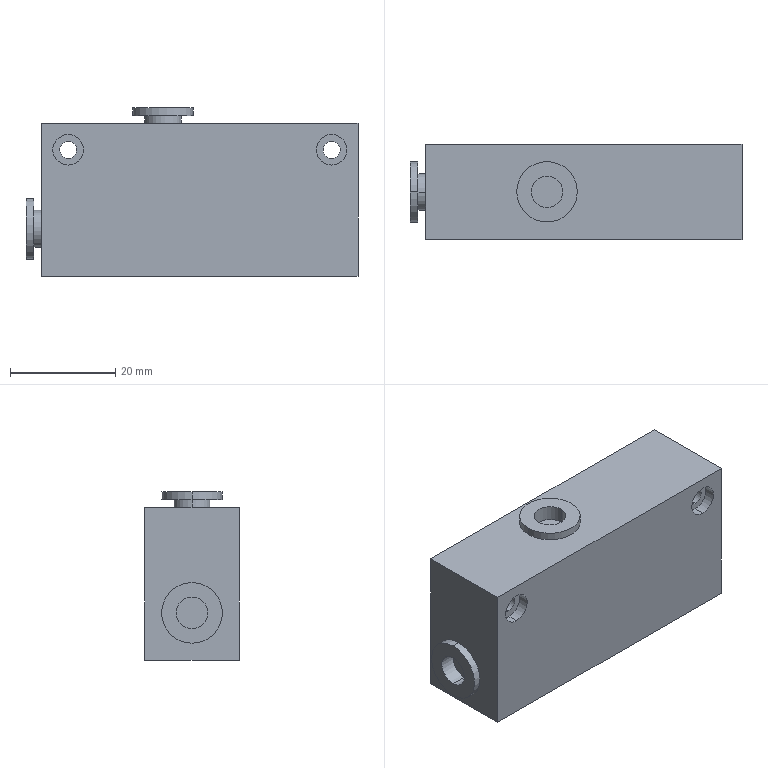Part | 1 solid | 40 faces | box 63 x 18 x 32 mm | volume 31141 mm3 | cylinder 24 | plane 16 | commonest cylinder face diameters 5.8 x8 3.2 x4 6 x4 7 x4 11.5 x4
STEP:
#1=CARTESIAN_POINT('',(32.,7.,12.1));
#2=VERTEX_POINT('',#1);
#3=CARTESIAN_POINT('',(32.,7.,17.9));
#4=VERTEX_POINT('',#3);
#5=CARTESIAN_POINT('',(32.,7.,15.));
#6=DIRECTION('',(0.,1.,0.));
#7=DIRECTION('',(0.,0.,1.));
#8=AXIS2_PLACEMENT_3D('',#5,#6,#7);
#9=CIRCLE('',#8,2.9);
#10=EDGE_CURVE('',#2,#4,#9,.T.);
#11=ORIENTED_EDGE('',*,*,#10,.F.);
#12=CARTESIAN_POINT('',(32.,9.,12.1));
#13=VERTEX_POINT('',#12);
#14=CARTESIAN_POINT('',(32.,-9.,12.1));
#15=DIRECTION('',(0.,1.,0.));
#16=VECTOR('',#15,1000.);
#17=LINE('',#14,#16);
#18=EDGE_CURVE('',#2,#13,#17,.T.);
#19=ORIENTED_EDGE('',*,*,#18,.T.);
#20=CARTESIAN_POINT('',(32.,9.,17.9));
#21=VERTEX_POINT('',#20);
#22=CARTESIAN_POINT('',(32.,9.,15.));
#23=DIRECTION('',(0.,-1.,0.));
#24=DIRECTION('',(0.,0.,1.));
#25=AXIS2_PLACEMENT_3D('',#22,#23,#24);
#26=CIRCLE('',#25,2.9);
#27=EDGE_CURVE('',#21,#13,#26,.T.);
#28=ORIENTED_EDGE('',*,*,#27,.F.);
#29=CARTESIAN_POINT('',(32.,-9.,17.9));
#30=DIRECTION('',(0.,1.,0.));
#31=VECTOR('',#30,1000.);
#32=LINE('',#29,#31);
#33=EDGE_CURVE('',#4,#21,#32,.T.);
#34=ORIENTED_EDGE('',*,*,#33,.F.);
#35=EDGE_LOOP('',(#11,#19,#28,#34));
#36=FACE_OUTER_BOUND('',#35,.T.);
#37=CARTESIAN_POINT('',(32.,-9.,15.));
#38=DIRECTION('',(0.,1.,0.));
#39=DIRECTION('',(0.,0.,1.));
#40=AXIS2_PLACEMENT_3D('',#37,#38,#39);
#41=CYLINDRICAL_SURFACE('',#40,2.9);
#42=ADVANCED_FACE('',(#36),#41,.F.);
#43=CARTESIAN_POINT('',(-18.,7.,12.1));
#44=VERTEX_POINT('',#43);
#45=CARTESIAN_POINT('',(-18.,7.,17.9));
#46=VERTEX_POINT('',#45);
#47=CARTESIAN_POINT('',(-18.,7.,15.));
#48=DIRECTION('',(0.,1.,0.));
#49=DIRECTION('',(0.,0.,1.));
#50=AXIS2_PLACEMENT_3D('',#47,#48,#49);
#51=CIRCLE('',#50,2.9);
#52=EDGE_CURVE('',#44,#46,#51,.T.);
#53=ORIENTED_EDGE('',*,*,#52,.F.);
#54=CARTESIAN_POINT('',(-18.,9.,12.1));
#55=VERTEX_POINT('',#54);
#56=CARTESIAN_POINT('',(-18.,-9.,12.1));
#57=DIRECTION('',(0.,1.,0.));
#58=VECTOR('',#57,1000.);
#59=LINE('',#56,#58);
#60=EDGE_CURVE('',#44,#55,#59,.T.);
#61=ORIENTED_EDGE('',*,*,#60,.T.);
#62=CARTESIAN_POINT('',(-18.,9.,17.9));
#63=VERTEX_POINT('',#62);
#64=CARTESIAN_POINT('',(-18.,9.,15.));
#65=DIRECTION('',(0.,-1.,0.));
#66=DIRECTION('',(0.,0.,1.));
#67=AXIS2_PLACEMENT_3D('',#64,#65,#66);
#68=CIRCLE('',#67,2.9);
#69=EDGE_CURVE('',#63,#55,#68,.T.);
#70=ORIENTED_EDGE('',*,*,#69,.F.);
#71=CARTESIAN_POINT('',(-18.,-9.,17.9));
#72=DIRECTION('',(0.,1.,0.));
#73=VECTOR('',#72,1000.);
#74=LINE('',#71,#73);
#75=EDGE_CURVE('',#46,#63,#74,.T.);
#76=ORIENTED_EDGE('',*,*,#75,.F.);
#77=EDGE_LOOP('',(#53,#61,#70,#76));
#78=FACE_OUTER_BOUND('',#77,.T.);
#79=CARTESIAN_POINT('',(-18.,-9.,15.));
#80=DIRECTION('',(0.,1.,0.));
#81=DIRECTION('',(0.,0.,1.));
#82=AXIS2_PLACEMENT_3D('',#79,#80,#81);
#83=CYLINDRICAL_SURFACE('',#82,2.9);
#84=ADVANCED_FACE('',(#78),#83,.F.);
#85=CARTESIAN_POINT('',(-3.5,0.,21.499));
#86=VERTEX_POINT('',#85);
#87=CARTESIAN_POINT('',(3.5,0.,21.499));
#88=VERTEX_POINT('',#87);
#89=CARTESIAN_POINT('',(0.,0.,21.499));
#90=DIRECTION('',(0.,0.,-1.));
#91=DIRECTION('',(-1.,0.,0.));
#92=AXIS2_PLACEMENT_3D('',#89,#90,#91);
#93=CIRCLE('',#92,3.5);
#94=EDGE_CURVE('',#86,#88,#93,.T.);
#95=ORIENTED_EDGE('',*,*,#94,.T.);
#96=CARTESIAN_POINT('',(3.5,0.,19.999));
#97=VERTEX_POINT('',#96);
#98=CARTESIAN_POINT('',(3.5,0.,50.));
#99=DIRECTION('',(0.,0.,-1.));
#100=VECTOR('',#99,1000.);
#101=LINE('',#98,#100);
#102=EDGE_CURVE('',#88,#97,#101,.T.);
#103=ORIENTED_EDGE('',*,*,#102,.T.);
#104=CARTESIAN_POINT('',(-3.5,0.,19.999));
#105=VERTEX_POINT('',#104);
#106=CARTESIAN_POINT('',(0.,0.,19.999));
#107=DIRECTION('',(0.,0.,1.));
#108=DIRECTION('',(-1.,0.,0.));
#109=AXIS2_PLACEMENT_3D('',#106,#107,#108);
#110=CIRCLE('',#109,3.5);
#111=EDGE_CURVE('',#97,#105,#110,.T.);
#112=ORIENTED_EDGE('',*,*,#111,.T.);
#113=CARTESIAN_POINT('',(-3.5,0.,50.));
#114=DIRECTION('',(0.,0.,-1.));
#115=VECTOR('',#114,1000.);
#116=LINE('',#113,#115);
#117=EDGE_CURVE('',#86,#105,#116,.T.);
#118=ORIENTED_EDGE('',*,*,#117,.F.);
#119=EDGE_LOOP('',(#95,#103,#112,#118));
#120=FACE_OUTER_BOUND('',#119,.T.);
#121=CARTESIAN_POINT('',(0.,0.,50.));
#122=DIRECTION('',(0.,0.,-1.));
#123=DIRECTION('',(-1.,0.,0.));
#124=AXIS2_PLACEMENT_3D('',#121,#122,#123);
#125=CYLINDRICAL_SURFACE('',#124,3.5);
#126=ADVANCED_FACE('',(#120),#125,.T.);
#127=CARTESIAN_POINT('',(-23.,0.,3.5));
#128=VERTEX_POINT('',#127);
#129=CARTESIAN_POINT('',(-23.,0.,-3.5));
#130=VERTEX_POINT('',#129);
#131=CARTESIAN_POINT('',(-23.,0.,0.));
#132=DIRECTION('',(-1.,0.,0.));
#133=DIRECTION('',(0.,0.,1.));
#134=AXIS2_PLACEMENT_3D('',#131,#132,#133);
#135=CIRCLE('',#134,3.5);
#136=EDGE_CURVE('',#128,#130,#135,.T.);
#137=ORIENTED_EDGE('',*,*,#136,.T.);
#138=CARTESIAN_POINT('',(-24.5,0.,-3.5));
#139=VERTEX_POINT('',#138);
#140=CARTESIAN_POINT('',(24.,0.,-3.5));
#141=DIRECTION('',(-1.,0.,0.));
#142=VECTOR('',#141,1000.);
#143=LINE('',#140,#142);
#144=EDGE_CURVE('',#130,#139,#143,.T.);
#145=ORIENTED_EDGE('',*,*,#144,.T.);
#146=CARTESIAN_POINT('',(-24.5,0.,3.5));
#147=VERTEX_POINT('',#146);
#148=CARTESIAN_POINT('',(-24.5,0.,0.));
#149=DIRECTION('',(1.,0.,0.));
#150=DIRECTION('',(0.,0.,1.));
#151=AXIS2_PLACEMENT_3D('',#148,#149,#150);
#152=CIRCLE('',#151,3.5);
#153=EDGE_CURVE('',#139,#147,#152,.T.);
#154=ORIENTED_EDGE('',*,*,#153,.T.);
#155=CARTESIAN_POINT('',(24.,0.,3.5));
#156=DIRECTION('',(-1.,0.,0.));
#157=VECTOR('',#156,1000.);
#158=LINE('',#155,#157);
#159=EDGE_CURVE('',#128,#147,#158,.T.);
#160=ORIENTED_EDGE('',*,*,#159,.F.);
#161=EDGE_LOOP('',(#137,#145,#154,#160));
#162=FACE_OUTER_BOUND('',#161,.T.);
#163=CARTESIAN_POINT('',(24.,0.,0.));
#164=DIRECTION('',(-1.,0.,0.));
#165=DIRECTION('',(0.,0.,1.));
#166=AXIS2_PLACEMENT_3D('',#163,#164,#165);
#167=CYLINDRICAL_SURFACE('',#166,3.5);
#168=ADVANCED_FACE('',(#162),#167,.T.);
#169=CARTESIAN_POINT('',(32.,-7.,13.4));
#170=VERTEX_POINT('',#169);
#171=CARTESIAN_POINT('',(32.,-7.,16.6));
#172=VERTEX_POINT('',#171);
#173=CARTESIAN_POINT('',(32.,-7.,15.));
#174=DIRECTION('',(0.,1.,0.));
#175=DIRECTION('',(0.,0.,1.));
#176=AXIS2_PLACEMENT_3D('',#173,#174,#175);
#177=CIRCLE('',#176,1.6);
#178=EDGE_CURVE('',#170,#172,#177,.T.);
#179=ORIENTED_EDGE('',*,*,#178,.F.);
#180=CARTESIAN_POINT('',(32.,7.,13.4));
#181=VERTEX_POINT('',#180);
#182=CARTESIAN_POINT('',(32.,-9.,13.4));
#183=DIRECTION('',(0.,1.,0.));
#184=VECTOR('',#183,1000.);
#185=LINE('',#182,#184);
#186=EDGE_CURVE('',#170,#181,#185,.T.);
#187=ORIENTED_EDGE('',*,*,#186,.T.);
#188=CARTESIAN_POINT('',(32.,7.,16.6));
#189=VERTEX_POINT('',#188);
#190=CARTESIAN_POINT('',(32.,7.,15.));
#191=DIRECTION('',(0.,-1.,0.));
#192=DIRECTION('',(0.,0.,1.));
#193=AXIS2_PLACEMENT_3D('',#190,#191,#192);
#194=CIRCLE('',#193,1.6);
#195=EDGE_CURVE('',#189,#181,#194,.T.);
#196=ORIENTED_EDGE('',*,*,#195,.F.);
#197=CARTESIAN_POINT('',(32.,-9.,16.6));
#198=DIRECTION('',(0.,1.,0.));
#199=VECTOR('',#198,1000.);
#200=LINE('',#197,#199);
#201=EDGE_CURVE('',#172,#189,#200,.T.);
#202=ORIENTED_EDGE('',*,*,#201,.F.);
#203=EDGE_LOOP('',(#179,#187,#196,#202));
#204=FACE_OUTER_BOUND('',#203,.T.);
#205=CARTESIAN_POINT('',(32.,-9.,15.));
#206=DIRECTION('',(0.,1.,0.));
#207=DIRECTION('',(0.,0.,1.));
#208=AXIS2_PLACEMENT_3D('',#205,#206,#207);
#209=CYLINDRICAL_SURFACE('',#208,1.6);
#210=ADVANCED_FACE('',(#204),#209,.F.);
#211=CARTESIAN_POINT('',(32.,-9.,17.9));
#212=VERTEX_POINT('',#211);
#213=CARTESIAN_POINT('',(32.,-9.,12.1));
#214=VERTEX_POINT('',#213);
#215=CARTESIAN_POINT('',(32.,-9.,15.));
#216=DIRECTION('',(0.,-1.,0.));
#217=DIRECTION('',(0.,0.,1.));
#218=AXIS2_PLACEMENT_3D('',#215,#216,#217);
#219=CIRCLE('',#218,2.9);
#220=EDGE_CURVE('',#212,#214,#219,.T.);
#221=ORIENTED_EDGE('',*,*,#220,.T.);
#222=CARTESIAN_POINT('',(32.,-7.,12.1));
#223=VERTEX_POINT('',#222);
#224=CARTESIAN_POINT('',(32.,-9.,12.1));
#225=DIRECTION('',(0.,1.,0.));
#226=VECTOR('',#225,1000.);
#227=LINE('',#224,#226);
#228=EDGE_CURVE('',#214,#223,#227,.T.);
#229=ORIENTED_EDGE('',*,*,#228,.T.);
#230=CARTESIAN_POINT('',(32.,-7.,17.9));
#231=VERTEX_POINT('',#230);
#232=CARTESIAN_POINT('',(32.,-7.,15.));
#233=DIRECTION('',(0.,-1.,0.));
#234=DIRECTION('',(0.,0.,1.));
#235=AXIS2_PLACEMENT_3D('',#232,#233,#234);
#236=CIRCLE('',#235,2.9);
#237=EDGE_CURVE('',#231,#223,#236,.T.);
#238=ORIENTED_EDGE('',*,*,#237,.F.);
#239=CARTESIAN_POINT('',(32.,-9.,17.9));
#240=DIRECTION('',(0.,1.,0.));
#241=VECTOR('',#240,1000.);
#242=LINE('',#239,#241);
#243=EDGE_CURVE('',#212,#231,#242,.T.);
#244=ORIENTED_EDGE('',*,*,#243,.F.);
#245=EDGE_LOOP('',(#221,#229,#238,#244));
#246=FACE_OUTER_BOUND('',#245,.T.);
#247=CARTESIAN_POINT('',(32.,-9.,15.));
#248=DIRECTION('',(0.,1.,0.));
#249=DIRECTION('',(0.,0.,1.));
#250=AXIS2_PLACEMENT_3D('',#247,#248,#249);
#251=CYLINDRICAL_SURFACE('',#250,2.9);
#252=ADVANCED_FACE('',(#246),#251,.F.);
#253=CARTESIAN_POINT('',(-18.,-9.,17.9));
#254=VERTEX_POINT('',#253);
#255=CARTESIAN_POINT('',(-18.,-9.,12.1));
#256=VERTEX_POINT('',#255);
#257=CARTESIAN_POINT('',(-18.,-9.,15.));
#258=DIRECTION('',(0.,-1.,0.));
#259=DIRECTION('',(0.,0.,1.));
#260=AXIS2_PLACEMENT_3D('',#257,#258,#259);
#261=CIRCLE('',#260,2.9);
#262=EDGE_CURVE('',#254,#256,#261,.T.);
#263=ORIENTED_EDGE('',*,*,#262,.T.);
#264=CARTESIAN_POINT('',(-18.,-7.,12.1));
#265=VERTEX_POINT('',#264);
#266=CARTESIAN_POINT('',(-18.,-9.,12.1));
#267=DIRECTION('',(0.,1.,0.));
#268=VECTOR('',#267,1000.);
#269=LINE('',#266,#268);
#270=EDGE_CURVE('',#256,#265,#269,.T.);
#271=ORIENTED_EDGE('',*,*,#270,.T.);
#272=CARTESIAN_POINT('',(-18.,-7.,17.9));
#273=VERTEX_POINT('',#272);
#274=CARTESIAN_POINT('',(-18.,-7.,15.));
#275=DIRECTION('',(0.,-1.,0.));
#276=DIRECTION('',(0.,0.,1.));
#277=AXIS2_PLACEMENT_3D('',#274,#275,#276);
#278=CIRCLE('',#277,2.9);
#279=EDGE_CURVE('',#273,#265,#278,.T.);
#280=ORIENTED_EDGE('',*,*,#279,.F.);
#281=CARTESIAN_POINT('',(-18.,-9.,17.9));
#282=DIRECTION('',(0.,1.,0.));
#283=VECTOR('',#282,1000.);
#284=LINE('',#281,#283);
#285=EDGE_CURVE('',#254,#273,#284,.T.);
#286=ORIENTED_EDGE('',*,*,#285,.F.);
#287=EDGE_LOOP('',(#263,#271,#280,#286));
#288=FACE_OUTER_BOUND('',#287,.T.);
#289=CARTESIAN_POINT('',(-18.,-9.,15.));
#290=DIRECTION('',(0.,1.,0.));
#291=DIRECTION('',(0.,0.,1.));
#292=AXIS2_PLACEMENT_3D('',#289,#290,#291);
#293=CYLINDRICAL_SURFACE('',#292,2.9);
#294=ADVANCED_FACE('',(#288),#293,.F.);
#295=CARTESIAN_POINT('',(-18.,-7.,13.4));
#296=VERTEX_POINT('',#295);
#297=CARTESIAN_POINT('',(-18.,-7.,16.6));
#298=VERTEX_POINT('',#297);
#299=CARTESIAN_POINT('',(-18.,-7.,15.));
#300=DIRECTION('',(0.,1.,0.));
#301=DIRECTION('',(0.,0.,1.));
#302=AXIS2_PLACEMENT_3D('',#299,#300,#301);
#303=CIRCLE('',#302,1.6);
#304=EDGE_CURVE('',#296,#298,#303,.T.);
#305=ORIENTED_EDGE('',*,*,#304,.F.);
#306=CARTESIAN_POINT('',(-18.,7.,13.4));
#307=VERTEX_POINT('',#306);
#308=CARTESIAN_POINT('',(-18.,-9.,13.4));
#309=DIRECTION('',(0.,1.,0.));
#310=VECTOR('',#309,1000.);
#311=LINE('',#308,#310);
#312=EDGE_CURVE('',#296,#307,#311,.T.);
#313=ORIENTED_EDGE('',*,*,#312,.T.);
#314=CARTESIAN_POINT('',(-18.,7.,16.6));
#315=VERTEX_POINT('',#314);
#316=CARTESIAN_POINT('',(-18.,7.,15.));
#317=DIRECTION('',(0.,-1.,0.));
#318=DIRECTION('',(0.,0.,1.));
#319=AXIS2_PLACEMENT_3D('',#316,#317,#318);
#320=CIRCLE('',#319,1.6);
#321=EDGE_CURVE('',#315,#307,#320,.T.);
#322=ORIENTED_EDGE('',*,*,#321,.F.);
#323=CARTESIAN_POINT('',(-18.,-9.,16.6));
#324=DIRECTION('',(0.,1.,0.));
#325=VECTOR('',#324,1000.);
#326=LINE('',#323,#325);
#327=EDGE_CURVE('',#298,#315,#326,.T.);
#328=ORIENTED_EDGE('',*,*,#327,.F.);
#329=EDGE_LOOP('',(#305,#313,#322,#328));
#330=FACE_OUTER_BOUND('',#329,.T.);
#331=CARTESIAN_POINT('',(-18.,-9.,15.));
#332=DIRECTION('',(0.,1.,0.));
#333=DIRECTION('',(0.,0.,1.));
#334=AXIS2_PLACEMENT_3D('',#331,#332,#333);
#335=CYLINDRICAL_SURFACE('',#334,1.6);
#336=ADVANCED_FACE('',(#330),#335,.F.);
#337=CARTESIAN_POINT('',(-5.75,0.,22.999));
#338=VERTEX_POINT('',#337);
#339=CARTESIAN_POINT('',(5.75,0.,22.999));
#340=VERTEX_POINT('',#339);
#341=CARTESIAN_POINT('',(0.,0.,22.999));
#342=DIRECTION('',(0.,0.,-1.));
#343=DIRECTION('',(-1.,0.,0.));
#344=AXIS2_PLACEMENT_3D('',#341,#342,#343);
#345=CIRCLE('',#344,5.75);
#346=EDGE_CURVE('',#338,#340,#345,.T.);
#347=ORIENTED_EDGE('',*,*,#346,.T.);
#348=CARTESIAN_POINT('',(5.75,0.,21.499));
#349=VERTEX_POINT('',#348);
#350=CARTESIAN_POINT('',(5.75,0.,50.));
#351=DIRECTION('',(0.,0.,-1.));
#352=VECTOR('',#351,1000.);
#353=LINE('',#350,#352);
#354=EDGE_CURVE('',#340,#349,#353,.T.);
#355=ORIENTED_EDGE('',*,*,#354,.T.);
#356=CARTESIAN_POINT('',(-5.75,0.,21.499));
#357=VERTEX_POINT('',#356);
#358=CARTESIAN_POINT('',(0.,0.,21.499));
#359=DIRECTION('',(0.,0.,-1.));
#360=DIRECTION('',(-1.,0.,0.));
#361=AXIS2_PLACEMENT_3D('',#358,#359,#360);
#362=CIRCLE('',#361,5.75);
#363=EDGE_CURVE('',#357,#349,#362,.T.);
#364=ORIENTED_EDGE('',*,*,#363,.F.);
#365=CARTESIAN_POINT('',(-5.75,0.,50.));
#366=DIRECTION('',(0.,0.,-1.));
#367=VECTOR('',#366,1000.);
#368=LINE('',#365,#367);
#369=EDGE_CURVE('',#338,#357,#368,.T.);
#370=ORIENTED_EDGE('',*,*,#369,.F.);
#371=EDGE_LOOP('',(#347,#355,#364,#370));
#372=FACE_OUTER_BOUND('',#371,.T.);
#373=CARTESIAN_POINT('',(0.,0.,50.));
#374=DIRECTION('',(0.,0.,-1.));
#375=DIRECTION('',(-1.,0.,0.));
#376=AXIS2_PLACEMENT_3D('',#373,#374,#375);
#377=CYLINDRICAL_SURFACE('',#376,5.75);
#378=ADVANCED_FACE('',(#372),#377,.T.);
#379=CARTESIAN_POINT('',(-24.5,0.,-5.75));
#380=VERTEX_POINT('',#379);
#381=CARTESIAN_POINT('',(-24.5,0.,5.75));
#382=VERTEX_POINT('',#381);
#383=CARTESIAN_POINT('',(-24.5,0.,0.));
#384=DIRECTION('',(1.,0.,0.));
#385=DIRECTION('',(0.,0.,1.));
#386=AXIS2_PLACEMENT_3D('',#383,#384,#385);
#387=CIRCLE('',#386,5.75);
#388=EDGE_CURVE('',#380,#382,#387,.T.);
#389=ORIENTED_EDGE('',*,*,#388,.F.);
#390=CARTESIAN_POINT('',(-26.,0.,-5.75));
#391=VERTEX_POINT('',#390);
#392=CARTESIAN_POINT('',(24.,0.,-5.75));
#393=DIRECTION('',(-1.,0.,0.));
#394=VECTOR('',#393,1000.);
#395=LINE('',#392,#394);
#396=EDGE_CURVE('',#380,#391,#395,.T.);
#397=ORIENTED_EDGE('',*,*,#396,.T.);
#398=CARTESIAN_POINT('',(-26.,0.,5.75));
#399=VERTEX_POINT('',#398);
#400=CARTESIAN_POINT('',(-26.,0.,0.));
#401=DIRECTION('',(1.,0.,0.));
#402=DIRECTION('',(0.,0.,1.));
#403=AXIS2_PLACEMENT_3D('',#400,#401,#402);
#404=CIRCLE('',#403,5.75);
#405=EDGE_CURVE('',#391,#399,#404,.T.);
#406=ORIENTED_EDGE('',*,*,#405,.T.);
#407=CARTESIAN_POINT('',(24.,0.,5.75));
#408=DIRECTION('',(-1.,0.,0.));
#409=VECTOR('',#408,1000.);
#410=LINE('',#407,#409);
#411=EDGE_CURVE('',#382,#399,#410,.T.);
#412=ORIENTED_EDGE('',*,*,#411,.F.);
#413=EDGE_LOOP('',(#389,#397,#406,#412));
#414=FACE_OUTER_BOUND('',#413,.T.);
#415=CARTESIAN_POINT('',(24.,0.,0.));
#416=DIRECTION('',(-1.,0.,0.));
#417=DIRECTION('',(0.,0.,1.));
#418=AXIS2_PLACEMENT_3D('',#415,#416,#417);
#419=CYLINDRICAL_SURFACE('',#418,5.75);
#420=ADVANCED_FACE('',(#414),#419,.T.);
#421=CARTESIAN_POINT('',(3.,0.,22.999));
#422=VERTEX_POINT('',#421);
#423=CARTESIAN_POINT('',(-3.,0.,22.999));
#424=VERTEX_POINT('',#423);
#425=CARTESIAN_POINT('',(0.,0.,22.999));
#426=DIRECTION('',(0.,0.,-1.));
#427=DIRECTION('',(-1.,0.,0.));
#428=AXIS2_PLACEMENT_3D('',#425,#426,#427);
#429=CIRCLE('',#428,3.);
#430=EDGE_CURVE('',#422,#424,#429,.T.);
#431=ORIENTED_EDGE('',*,*,#430,.F.);
#432=CARTESIAN_POINT('',(3.,0.,19.999));
#433=VERTEX_POINT('',#432);
#434=CARTESIAN_POINT('',(3.,0.,50.));
#435=DIRECTION('',(0.,0.,-1.));
#436=VECTOR('',#435,1000.);
#437=LINE('',#434,#436);
#438=EDGE_CURVE('',#422,#433,#437,.T.);
#439=ORIENTED_EDGE('',*,*,#438,.T.);
#440=CARTESIAN_POINT('',(-3.,0.,19.999));
#441=VERTEX_POINT('',#440);
#442=CARTESIAN_POINT('',(0.,0.,19.999));
#443=DIRECTION('',(0.,0.,1.));
#444=DIRECTION('',(-1.,0.,0.));
#445=AXIS2_PLACEMENT_3D('',#442,#443,#444);
#446=CIRCLE('',#445,3.);
#447=EDGE_CURVE('',#441,#433,#446,.T.);
#448=ORIENTED_EDGE('',*,*,#447,.F.);
#449=CARTESIAN_POINT('',(-3.,0.,50.));
#450=DIRECTION('',(0.,0.,-1.));
#451=VECTOR('',#450,1000.);
#452=LINE('',#449,#451);
#453=EDGE_CURVE('',#424,#441,#452,.T.);
#454=ORIENTED_EDGE('',*,*,#453,.F.);
#455=EDGE_LOOP('',(#431,#439,#448,#454));
#456=FACE_OUTER_BOUND('',#455,.T.);
#457=CARTESIAN_POINT('',(0.,0.,50.));
#458=DIRECTION('',(0.,0.,-1.));
#459=DIRECTION('',(-1.,0.,0.));
#460=AXIS2_PLACEMENT_3D('',#457,#458,#459);
#461=CYLINDRICAL_SURFACE('',#460,3.);
#462=ADVANCED_FACE('',(#456),#461,.F.);
#463=CARTESIAN_POINT('',(-23.,0.,-3.));
#464=VERTEX_POINT('',#463);
#465=CARTESIAN_POINT('',(-23.,0.,3.));
#466=VERTEX_POINT('',#465);
#467=CARTESIAN_POINT('',(-23.,0.,0.));
#468=DIRECTION('',(-1.,0.,0.));
#469=DIRECTION('',(0.,0.,1.));
#470=AXIS2_PLACEMENT_3D('',#467,#468,#469);
#471=CIRCLE('',#470,3.);
#472=EDGE_CURVE('',#464,#466,#471,.T.);
#473=ORIENTED_EDGE('',*,*,#472,.F.);
#474=CARTESIAN_POINT('',(-26.,0.,-3.));
#475=VERTEX_POINT('',#474);
#476=CARTESIAN_POINT('',(24.,0.,-3.));
#477=DIRECTION('',(-1.,0.,0.));
#478=VECTOR('',#477,1000.);
#479=LINE('',#476,#478);
#480=EDGE_CURVE('',#464,#475,#479,.T.);
#481=ORIENTED_EDGE('',*,*,#480,.T.);
#482=CARTESIAN_POINT('',(-26.,0.,3.));
#483=VERTEX_POINT('',#482);
#484=CARTESIAN_POINT('',(-26.,0.,0.));
#485=DIRECTION('',(1.,0.,0.));
#486=DIRECTION('',(0.,0.,1.));
#487=AXIS2_PLACEMENT_3D('',#484,#485,#486);
#488=CIRCLE('',#487,3.);
#489=EDGE_CURVE('',#483,#475,#488,.T.);
#490=ORIENTED_EDGE('',*,*,#489,.F.);
#491=CARTESIAN_POINT('',(24.,0.,3.));
#492=DIRECTION('',(-1.,0.,0.));
#493=VECTOR('',#492,1000.);
#494=LINE('',#491,#493);
#495=EDGE_CURVE('',#466,#483,#494,.T.);
#496=ORIENTED_EDGE('',*,*,#495,.F.);
#497=EDGE_LOOP('',(#473,#481,#490,#496));
#498=FACE_OUTER_BOUND('',#497,.T.);
#499=CARTESIAN_POINT('',(24.,0.,0.));
#500=DIRECTION('',(-1.,0.,0.));
#501=DIRECTION('',(0.,0.,1.));
#502=AXIS2_PLACEMENT_3D('',#499,#500,#501);
#503=CYLINDRICAL_SURFACE('',#502,3.);
#504=ADVANCED_FACE('',(#498),#503,.F.);
#505=ORIENTED_EDGE('',*,*,#27,.T.);
#506=CARTESIAN_POINT('',(32.,9.,15.));
#507=DIRECTION('',(0.,-1.,0.));
#508=DIRECTION('',(0.,0.,1.));
#509=AXIS2_PLACEMENT_3D('',#506,#507,#508);
#510=CIRCLE('',#509,2.9);
#511=EDGE_CURVE('',#13,#21,#510,.T.);
#512=ORIENTED_EDGE('',*,*,#511,.T.);
#513=EDGE_LOOP('',(#505,#512));
#514=FACE_BOUND('',#513,.T.);
#515=CARTESIAN_POINT('',(37.,9.,19.999));
#516=VERTEX_POINT('',#515);
#517=CARTESIAN_POINT('',(37.,9.,-9.001));
#518=VERTEX_POINT('',#517);
#519=CARTESIAN_POINT('',(37.,9.,0.));
#520=DIRECTION('',(0.,0.,-1.));
#521=VECTOR('',#520,1000.);
#522=LINE('',#519,#521);
#523=EDGE_CURVE('',#516,#518,#522,.T.);
#524=ORIENTED_EDGE('',*,*,#523,.T.);
#525=CARTESIAN_POINT('',(-23.,9.,-9.001));
#526=VERTEX_POINT('',#525);
#527=CARTESIAN_POINT('',(0.,9.,-9.001));
#528=DIRECTION('',(-1.,0.,0.));
#529=VECTOR('',#528,1000.);
#530=LINE('',#527,#529);
#531=EDGE_CURVE('',#518,#526,#530,.T.);
#532=ORIENTED_EDGE('',*,*,#531,.T.);
#533=CARTESIAN_POINT('',(-23.,9.,19.999));
#534=VERTEX_POINT('',#533);
#535=CARTESIAN_POINT('',(-23.,9.,0.));
#536=DIRECTION('',(0.,0.,1.));
#537=VECTOR('',#536,1000.);
#538=LINE('',#535,#537);
#539=EDGE_CURVE('',#526,#534,#538,.T.);
#540=ORIENTED_EDGE('',*,*,#539,.T.);
#541=CARTESIAN_POINT('',(0.,9.,19.999));
#542=DIRECTION('',(1.,0.,0.));
#543=VECTOR('',#542,1000.);
#544=LINE('',#541,#543);
#545=EDGE_CURVE('',#534,#516,#544,.T.);
#546=ORIENTED_EDGE('',*,*,#545,.T.);
#547=EDGE_LOOP('',(#524,#532,#540,#546));
#548=FACE_OUTER_BOUND('',#547,.T.);
#549=ORIENTED_EDGE('',*,*,#69,.T.);
#550=CARTESIAN_POINT('',(-18.,9.,15.));
#551=DIRECTION('',(0.,-1.,0.));
#552=DIRECTION('',(0.,0.,1.));
#553=AXIS2_PLACEMENT_3D('',#550,#551,#552);
#554=CIRCLE('',#553,2.9);
#555=EDGE_CURVE('',#55,#63,#554,.T.);
#556=ORIENTED_EDGE('',*,*,#555,.T.);
#557=EDGE_LOOP('',(#549,#556));
#558=FACE_BOUND('',#557,.T.);
#559=CARTESIAN_POINT('',(0.,9.,0.));
#560=DIRECTION('',(0.,1.,0.));
#561=DIRECTION('',(0.,0.,1.));
#562=AXIS2_PLACEMENT_3D('',#559,#560,#561);
#563=PLANE('',#562);
#564=ADVANCED_FACE('',(#514,#548,#558),#563,.T.);
#565=ORIENTED_EDGE('',*,*,#18,.F.);
#566=CARTESIAN_POINT('',(32.,7.,15.));
#567=DIRECTION('',(0.,1.,0.));
#568=DIRECTION('',(0.,0.,1.));
#569=AXIS2_PLACEMENT_3D('',#566,#567,#568);
#570=CIRCLE('',#569,2.9);
#571=EDGE_CURVE('',#4,#2,#570,.T.);
#572=ORIENTED_EDGE('',*,*,#571,.F.);
#573=ORIENTED_EDGE('',*,*,#33,.T.);
#574=ORIENTED_EDGE('',*,*,#511,.F.);
#575=EDGE_LOOP('',(#565,#572,#573,#574));
#576=FACE_OUTER_BOUND('',#575,.T.);
#577=CARTESIAN_POINT('',(32.,-9.,15.));
#578=DIRECTION('',(0.,1.,0.));
#579=DIRECTION('',(0.,0.,1.));
#580=AXIS2_PLACEMENT_3D('',#577,#578,#579);
#581=CYLINDRICAL_SURFACE('',#580,2.9);
#582=ADVANCED_FACE('',(#576),#581,.F.);
#583=CARTESIAN_POINT('',(-23.,-9.,-9.001));
#584=VERTEX_POINT('',#583);
#585=CARTESIAN_POINT('',(-23.,9.,-9.001));
#586=DIRECTION('',(0.,-1.,0.));
#587=VECTOR('',#586,1000.);
#588=LINE('',#585,#587);
#589=EDGE_CURVE('',#526,#584,#588,.T.);
#590=ORIENTED_EDGE('',*,*,#589,.F.);
#591=ORIENTED_EDGE('',*,*,#531,.F.);
#592=CARTESIAN_POINT('',(37.,-9.,-9.001));
#593=VERTEX_POINT('',#592);
#594=CARTESIAN_POINT('',(37.,9.,-9.001));
#595=DIRECTION('',(0.,1.,0.));
#596=VECTOR('',#595,1000.);
#597=LINE('',#594,#596);
#598=EDGE_CURVE('',#593,#518,#597,.T.);
#599=ORIENTED_EDGE('',*,*,#598,.F.);
#600=CARTESIAN_POINT('',(37.,-9.,-9.001));
#601=DIRECTION('',(1.,0.,0.));
#602=VECTOR('',#601,1000.);
#603=LINE('',#600,#602);
#604=EDGE_CURVE('',#584,#593,#603,.T.);
#605=ORIENTED_EDGE('',*,*,#604,.F.);
#606=EDGE_LOOP('',(#590,#591,#599,#605));
#607=FACE_OUTER_BOUND('',#606,.T.);
#608=CARTESIAN_POINT('',(37.,9.,-9.001));
#609=DIRECTION('',(0.,0.,1.));
#610=DIRECTION('',(1.,0.,0.));
#611=AXIS2_PLACEMENT_3D('',#608,#609,#610);
#612=PLANE('',#611);
#613=ADVANCED_FACE('',(#607),#612,.F.);
#614=ORIENTED_EDGE('',*,*,#598,.T.);
#615=ORIENTED_EDGE('',*,*,#523,.F.);
#616=CARTESIAN_POINT('',(37.,-9.,19.999));
#617=VERTEX_POINT('',#616);
#618=CARTESIAN_POINT('',(37.,9.,19.999));
#619=DIRECTION('',(0.,1.,0.));
#620=VECTOR('',#619,1000.);
#621=LINE('',#618,#620);
#622=EDGE_CURVE('',#617,#516,#621,.T.);
#623=ORIENTED_EDGE('',*,*,#622,.F.);
#624=CARTESIAN_POINT('',(37.,-9.,19.999));
#625=DIRECTION('',(0.,0.,1.));
#626=VECTOR('',#625,1000.);
#627=LINE('',#624,#626);
#628=EDGE_CURVE('',#593,#617,#627,.T.);
#629=ORIENTED_EDGE('',*,*,#628,.F.);
#630=EDGE_LOOP('',(#614,#615,#623,#629));
#631=FACE_OUTER_BOUND('',#630,.T.);
#632=CARTESIAN_POINT('',(37.,9.,19.999));
#633=DIRECTION('',(-1.,0.,0.));
#634=DIRECTION('',(0.,0.,1.));
#635=AXIS2_PLACEMENT_3D('',#632,#633,#634);
#636=PLANE('',#635);
#637=ADVANCED_FACE('',(#631),#636,.F.);
#638=ORIENTED_EDGE('',*,*,#622,.T.);
#639=ORIENTED_EDGE('',*,*,#545,.F.);
#640=CARTESIAN_POINT('',(-23.,-9.,19.999));
#641=VERTEX_POINT('',#640);
#642=CARTESIAN_POINT('',(-23.,9.,19.999));
#643=DIRECTION('',(0.,1.,0.));
#644=VECTOR('',#643,1000.);
#645=LINE('',#642,#644);
#646=EDGE_CURVE('',#641,#534,#645,.T.);
#647=ORIENTED_EDGE('',*,*,#646,.F.);
#648=CARTESIAN_POINT('',(-23.,-9.,19.999));
#649=DIRECTION('',(-1.,0.,0.));
#650=VECTOR('',#649,1000.);
#651=LINE('',#648,#650);
#652=EDGE_CURVE('',#617,#641,#651,.T.);
#653=ORIENTED_EDGE('',*,*,#652,.F.);
#654=EDGE_LOOP('',(#638,#639,#647,#653));
#655=FACE_OUTER_BOUND('',#654,.T.);
#656=CARTESIAN_POINT('',(0.,0.,19.999));
#657=DIRECTION('',(0.,0.,1.));
#658=DIRECTION('',(-1.,0.,0.));
#659=AXIS2_PLACEMENT_3D('',#656,#657,#658);
#660=CIRCLE('',#659,3.5);
#661=EDGE_CURVE('',#105,#97,#660,.T.);
#662=ORIENTED_EDGE('',*,*,#661,.F.);
#663=ORIENTED_EDGE('',*,*,#111,.F.);
#664=EDGE_LOOP('',(#662,#663));
#665=FACE_BOUND('',#664,.T.);
#666=CARTESIAN_POINT('',(-23.,9.,19.999));
#667=DIRECTION('',(0.,0.,-1.));
#668=DIRECTION('',(-1.,0.,0.));
#669=AXIS2_PLACEMENT_3D('',#666,#667,#668);
#670=PLANE('',#669);
#671=ADVANCED_FACE('',(#655,#665),#670,.F.);
#672=ORIENTED_EDGE('',*,*,#646,.T.);
#673=ORIENTED_EDGE('',*,*,#539,.F.);
#674=ORIENTED_EDGE('',*,*,#589,.T.);
#675=CARTESIAN_POINT('',(-23.,-9.,-9.001));
#676=DIRECTION('',(0.,0.,-1.));
#677=VECTOR('',#676,1000.);
#678=LINE('',#675,#677);
#679=EDGE_CURVE('',#641,#584,#678,.T.);
#680=ORIENTED_EDGE('',*,*,#679,.F.);
#681=EDGE_LOOP('',(#672,#673,#674,#680));
#682=FACE_OUTER_BOUND('',#681,.T.);
#683=ORIENTED_EDGE('',*,*,#136,.F.);
#684=CARTESIAN_POINT('',(-23.,0.,0.));
#685=DIRECTION('',(-1.,0.,0.));
#686=DIRECTION('',(0.,0.,1.));
#687=AXIS2_PLACEMENT_3D('',#684,#685,#686);
#688=CIRCLE('',#687,3.5);
#689=EDGE_CURVE('',#130,#128,#688,.T.);
#690=ORIENTED_EDGE('',*,*,#689,.F.);
#691=EDGE_LOOP('',(#683,#690));
#692=FACE_BOUND('',#691,.T.);
#693=CARTESIAN_POINT('',(-23.,9.,-9.001));
#694=DIRECTION('',(1.,0.,0.));
#695=DIRECTION('',(0.,0.,-1.));
#696=AXIS2_PLACEMENT_3D('',#693,#694,#695);
#697=PLANE('',#696);
#698=ADVANCED_FACE('',(#682,#692),#697,.F.);
#699=ORIENTED_EDGE('',*,*,#60,.F.);
#700=CARTESIAN_POINT('',(-18.,7.,15.));
#701=DIRECTION('',(0.,1.,0.));
#702=DIRECTION('',(0.,0.,1.));
#703=AXIS2_PLACEMENT_3D('',#700,#701,#702);
#704=CIRCLE('',#703,2.9);
#705=EDGE_CURVE('',#46,#44,#704,.T.);
#706=ORIENTED_EDGE('',*,*,#705,.F.);
#707=ORIENTED_EDGE('',*,*,#75,.T.);
#708=ORIENTED_EDGE('',*,*,#555,.F.);
#709=EDGE_LOOP('',(#699,#706,#707,#708));
#710=FACE_OUTER_BOUND('',#709,.T.);
#711=CARTESIAN_POINT('',(-18.,-9.,15.));
#712=DIRECTION('',(0.,1.,0.));
#713=DIRECTION('',(0.,0.,1.));
#714=AXIS2_PLACEMENT_3D('',#711,#712,#713);
#715=CYLINDRICAL_SURFACE('',#714,2.9);
#716=ADVANCED_FACE('',(#710),#715,.F.);
#717=ORIENTED_EDGE('',*,*,#571,.T.);
#718=ORIENTED_EDGE('',*,*,#10,.T.);
#719=EDGE_LOOP('',(#717,#718));
#720=FACE_OUTER_BOUND('',#719,.T.);
#721=ORIENTED_EDGE('',*,*,#195,.T.);
#722=CARTESIAN_POINT('',(32.,7.,15.));
#723=DIRECTION('',(0.,-1.,0.));
#724=DIRECTION('',(0.,0.,1.));
#725=AXIS2_PLACEMENT_3D('',#722,#723,#724);
#726=CIRCLE('',#725,1.6);
#727=EDGE_CURVE('',#181,#189,#726,.T.);
#728=ORIENTED_EDGE('',*,*,#727,.T.);
#729=EDGE_LOOP('',(#721,#728));
#730=FACE_BOUND('',#729,.T.);
#731=CARTESIAN_POINT('',(34.9,7.,15.));
#732=DIRECTION('',(0.,1.,0.));
#733=DIRECTION('',(0.,0.,1.));
#734=AXIS2_PLACEMENT_3D('',#731,#732,#733);
#735=PLANE('',#734);
#736=ADVANCED_FACE('',(#720,#730),#735,.T.);
#737=ORIENTED_EDGE('',*,*,#220,.F.);
#738=CARTESIAN_POINT('',(32.,-9.,15.));
#739=DIRECTION('',(0.,-1.,0.));
#740=DIRECTION('',(0.,0.,1.));
#741=AXIS2_PLACEMENT_3D('',#738,#739,#740);
#742=CIRCLE('',#741,2.9);
#743=EDGE_CURVE('',#214,#212,#742,.T.);
#744=ORIENTED_EDGE('',*,*,#743,.F.);
#745=EDGE_LOOP('',(#737,#744));
#746=FACE_BOUND('',#745,.T.);
#747=ORIENTED_EDGE('',*,*,#604,.T.);
#748=ORIENTED_EDGE('',*,*,#628,.T.);
#749=ORIENTED_EDGE('',*,*,#652,.T.);
#750=ORIENTED_EDGE('',*,*,#679,.T.);
#751=EDGE_LOOP('',(#747,#748,#749,#750));
#752=FACE_OUTER_BOUND('',#751,.T.);
#753=ORIENTED_EDGE('',*,*,#262,.F.);
#754=CARTESIAN_POINT('',(-18.,-9.,15.));
#755=DIRECTION('',(0.,-1.,0.));
#756=DIRECTION('',(0.,0.,1.));
#757=AXIS2_PLACEMENT_3D('',#754,#755,#756);
#758=CIRCLE('',#757,2.9);
#759=EDGE_CURVE('',#256,#254,#758,.T.);
#760=ORIENTED_EDGE('',*,*,#759,.F.);
#761=EDGE_LOOP('',(#753,#760));
#762=FACE_BOUND('',#761,.T.);
#763=CARTESIAN_POINT('',(0.,-9.,0.));
#764=DIRECTION('',(0.,1.,0.));
#765=DIRECTION('',(0.,0.,1.));
#766=AXIS2_PLACEMENT_3D('',#763,#764,#765);
#767=PLANE('',#766);
#768=ADVANCED_FACE('',(#746,#752,#762),#767,.F.);
#769=ORIENTED_EDGE('',*,*,#102,.F.);
#770=CARTESIAN_POINT('',(0.,0.,21.499));
#771=DIRECTION('',(0.,0.,-1.));
#772=DIRECTION('',(-1.,0.,0.));
#773=AXIS2_PLACEMENT_3D('',#770,#771,#772);
#774=CIRCLE('',#773,3.5);
#775=EDGE_CURVE('',#88,#86,#774,.T.);
#776=ORIENTED_EDGE('',*,*,#775,.T.);
#777=ORIENTED_EDGE('',*,*,#117,.T.);
#778=ORIENTED_EDGE('',*,*,#661,.T.);
#779=EDGE_LOOP('',(#769,#776,#777,#778));
#780=FACE_OUTER_BOUND('',#779,.T.);
#781=CARTESIAN_POINT('',(0.,0.,50.));
#782=DIRECTION('',(0.,0.,-1.));
#783=DIRECTION('',(-1.,0.,0.));
#784=AXIS2_PLACEMENT_3D('',#781,#782,#783);
#785=CYLINDRICAL_SURFACE('',#784,3.5);
#786=ADVANCED_FACE('',(#780),#785,.T.);
#787=ORIENTED_EDGE('',*,*,#144,.F.);
#788=ORIENTED_EDGE('',*,*,#689,.T.);
#789=ORIENTED_EDGE('',*,*,#159,.T.);
#790=CARTESIAN_POINT('',(-24.5,0.,0.));
#791=DIRECTION('',(1.,0.,0.));
#792=DIRECTION('',(0.,0.,1.));
#793=AXIS2_PLACEMENT_3D('',#790,#791,#792);
#794=CIRCLE('',#793,3.5);
#795=EDGE_CURVE('',#147,#139,#794,.T.);
#796=ORIENTED_EDGE('',*,*,#795,.T.);
#797=EDGE_LOOP('',(#787,#788,#789,#796));
#798=FACE_OUTER_BOUND('',#797,.T.);
#799=CARTESIAN_POINT('',(24.,0.,0.));
#800=DIRECTION('',(-1.,0.,0.));
#801=DIRECTION('',(0.,0.,1.));
#802=AXIS2_PLACEMENT_3D('',#799,#800,#801);
#803=CYLINDRICAL_SURFACE('',#802,3.5);
#804=ADVANCED_FACE('',(#798),#803,.T.);
#805=ORIENTED_EDGE('',*,*,#705,.T.);
#806=ORIENTED_EDGE('',*,*,#52,.T.);
#807=EDGE_LOOP('',(#805,#806));
#808=FACE_OUTER_BOUND('',#807,.T.);
#809=ORIENTED_EDGE('',*,*,#321,.T.);
#810=CARTESIAN_POINT('',(-18.,7.,15.));
#811=DIRECTION('',(0.,-1.,0.));
#812=DIRECTION('',(0.,0.,1.));
#813=AXIS2_PLACEMENT_3D('',#810,#811,#812);
#814=CIRCLE('',#813,1.6);
#815=EDGE_CURVE('',#307,#315,#814,.T.);
#816=ORIENTED_EDGE('',*,*,#815,.T.);
#817=EDGE_LOOP('',(#809,#816));
#818=FACE_BOUND('',#817,.T.);
#819=CARTESIAN_POINT('',(-15.1,7.,15.));
#820=DIRECTION('',(0.,1.,0.));
#821=DIRECTION('',(0.,0.,1.));
#822=AXIS2_PLACEMENT_3D('',#819,#820,#821);
#823=PLANE('',#822);
#824=ADVANCED_FACE('',(#808,#818),#823,.T.);
#825=ORIENTED_EDGE('',*,*,#186,.F.);
#826=CARTESIAN_POINT('',(32.,-7.,15.));
#827=DIRECTION('',(0.,1.,0.));
#828=DIRECTION('',(0.,0.,1.));
#829=AXIS2_PLACEMENT_3D('',#826,#827,#828);
#830=CIRCLE('',#829,1.6);
#831=EDGE_CURVE('',#172,#170,#830,.T.);
#832=ORIENTED_EDGE('',*,*,#831,.F.);
#833=ORIENTED_EDGE('',*,*,#201,.T.);
#834=ORIENTED_EDGE('',*,*,#727,.F.);
#835=EDGE_LOOP('',(#825,#832,#833,#834));
#836=FACE_OUTER_BOUND('',#835,.T.);
#837=CARTESIAN_POINT('',(32.,-9.,15.));
#838=DIRECTION('',(0.,1.,0.));
#839=DIRECTION('',(0.,0.,1.));
#840=AXIS2_PLACEMENT_3D('',#837,#838,#839);
#841=CYLINDRICAL_SURFACE('',#840,1.6);
#842=ADVANCED_FACE('',(#836),#841,.F.);
#843=ORIENTED_EDGE('',*,*,#228,.F.);
#844=ORIENTED_EDGE('',*,*,#743,.T.);
#845=ORIENTED_EDGE('',*,*,#243,.T.);
#846=CARTESIAN_POINT('',(32.,-7.,15.));
#847=DIRECTION('',(0.,-1.,0.));
#848=DIRECTION('',(0.,0.,1.));
#849=AXIS2_PLACEMENT_3D('',#846,#847,#848);
#850=CIRCLE('',#849,2.9);
#851=EDGE_CURVE('',#223,#231,#850,.T.);
#852=ORIENTED_EDGE('',*,*,#851,.F.);
#853=EDGE_LOOP('',(#843,#844,#845,#852));
#854=FACE_OUTER_BOUND('',#853,.T.);
#855=CARTESIAN_POINT('',(32.,-9.,15.));
#856=DIRECTION('',(0.,1.,0.));
#857=DIRECTION('',(0.,0.,1.));
#858=AXIS2_PLACEMENT_3D('',#855,#856,#857);
#859=CYLINDRICAL_SURFACE('',#858,2.9);
#860=ADVANCED_FACE('',(#854),#859,.F.);
#861=ORIENTED_EDGE('',*,*,#270,.F.);
#862=ORIENTED_EDGE('',*,*,#759,.T.);
#863=ORIENTED_EDGE('',*,*,#285,.T.);
#864=CARTESIAN_POINT('',(-18.,-7.,15.));
#865=DIRECTION('',(0.,-1.,0.));
#866=DIRECTION('',(0.,0.,1.));
#867=AXIS2_PLACEMENT_3D('',#864,#865,#866);
#868=CIRCLE('',#867,2.9);
#869=EDGE_CURVE('',#265,#273,#868,.T.);
#870=ORIENTED_EDGE('',*,*,#869,.F.);
#871=EDGE_LOOP('',(#861,#862,#863,#870));
#872=FACE_OUTER_BOUND('',#871,.T.);
#873=CARTESIAN_POINT('',(-18.,-9.,15.));
#874=DIRECTION('',(0.,1.,0.));
#875=DIRECTION('',(0.,0.,1.));
#876=AXIS2_PLACEMENT_3D('',#873,#874,#875);
#877=CYLINDRICAL_SURFACE('',#876,2.9);
#878=ADVANCED_FACE('',(#872),#877,.F.);
#879=ORIENTED_EDGE('',*,*,#363,.T.);
#880=CARTESIAN_POINT('',(0.,0.,21.499));
#881=DIRECTION('',(0.,0.,-1.));
#882=DIRECTION('',(-1.,0.,0.));
#883=AXIS2_PLACEMENT_3D('',#880,#881,#882);
#884=CIRCLE('',#883,5.75);
#885=EDGE_CURVE('',#349,#357,#884,.T.);
#886=ORIENTED_EDGE('',*,*,#885,.T.);
#887=EDGE_LOOP('',(#879,#886));
#888=FACE_OUTER_BOUND('',#887,.T.);
#889=ORIENTED_EDGE('',*,*,#94,.F.);
#890=ORIENTED_EDGE('',*,*,#775,.F.);
#891=EDGE_LOOP('',(#889,#890));
#892=FACE_BOUND('',#891,.T.);
#893=CARTESIAN_POINT('',(5.75,0.,21.499));
#894=DIRECTION('',(0.,0.,-1.));
#895=DIRECTION('',(-1.,0.,0.));
#896=AXIS2_PLACEMENT_3D('',#893,#894,#895);
#897=PLANE('',#896);
#898=ADVANCED_FACE('',(#888,#892),#897,.T.);
#899=ORIENTED_EDGE('',*,*,#795,.F.);
#900=ORIENTED_EDGE('',*,*,#153,.F.);
#901=EDGE_LOOP('',(#899,#900));
#902=FACE_BOUND('',#901,.T.);
#903=CARTESIAN_POINT('',(-24.5,0.,0.));
#904=DIRECTION('',(1.,0.,0.));
#905=DIRECTION('',(0.,0.,1.));
#906=AXIS2_PLACEMENT_3D('',#903,#904,#905);
#907=CIRCLE('',#906,5.75);
#908=EDGE_CURVE('',#382,#380,#907,.T.);
#909=ORIENTED_EDGE('',*,*,#908,.T.);
#910=ORIENTED_EDGE('',*,*,#388,.T.);
#911=EDGE_LOOP('',(#909,#910));
#912=FACE_OUTER_BOUND('',#911,.T.);
#913=CARTESIAN_POINT('',(-24.5,0.,-3.5));
#914=DIRECTION('',(1.,0.,0.));
#915=DIRECTION('',(0.,0.,-1.));
#916=AXIS2_PLACEMENT_3D('',#913,#914,#915);
#917=PLANE('',#916);
#918=ADVANCED_FACE('',(#902,#912),#917,.T.);
#919=ORIENTED_EDGE('',*,*,#312,.F.);
#920=CARTESIAN_POINT('',(-18.,-7.,15.));
#921=DIRECTION('',(0.,1.,0.));
#922=DIRECTION('',(0.,0.,1.));
#923=AXIS2_PLACEMENT_3D('',#920,#921,#922);
#924=CIRCLE('',#923,1.6);
#925=EDGE_CURVE('',#298,#296,#924,.T.);
#926=ORIENTED_EDGE('',*,*,#925,.F.);
#927=ORIENTED_EDGE('',*,*,#327,.T.);
#928=ORIENTED_EDGE('',*,*,#815,.F.);
#929=EDGE_LOOP('',(#919,#926,#927,#928));
#930=FACE_OUTER_BOUND('',#929,.T.);
#931=CARTESIAN_POINT('',(-18.,-9.,15.));
#932=DIRECTION('',(0.,1.,0.));
#933=DIRECTION('',(0.,0.,1.));
#934=AXIS2_PLACEMENT_3D('',#931,#932,#933);
#935=CYLINDRICAL_SURFACE('',#934,1.6);
#936=ADVANCED_FACE('',(#930),#935,.F.);
#937=ORIENTED_EDGE('',*,*,#831,.T.);
#938=ORIENTED_EDGE('',*,*,#178,.T.);
#939=EDGE_LOOP('',(#937,#938));
#940=FACE_BOUND('',#939,.T.);
#941=ORIENTED_EDGE('',*,*,#237,.T.);
#942=ORIENTED_EDGE('',*,*,#851,.T.);
#943=EDGE_LOOP('',(#941,#942));
#944=FACE_OUTER_BOUND('',#943,.T.);
#945=CARTESIAN_POINT('',(33.6,-7.,15.));
#946=DIRECTION('',(0.,-1.,0.));
#947=DIRECTION('',(0.,0.,-1.));
#948=AXIS2_PLACEMENT_3D('',#945,#946,#947);
#949=PLANE('',#948);
#950=ADVANCED_FACE('',(#940,#944),#949,.T.);
#951=ORIENTED_EDGE('',*,*,#925,.T.);
#952=ORIENTED_EDGE('',*,*,#304,.T.);
#953=EDGE_LOOP('',(#951,#952));
#954=FACE_BOUND('',#953,.T.);
#955=ORIENTED_EDGE('',*,*,#279,.T.);
#956=ORIENTED_EDGE('',*,*,#869,.T.);
#957=EDGE_LOOP('',(#955,#956));
#958=FACE_OUTER_BOUND('',#957,.T.);
#959=CARTESIAN_POINT('',(-16.4,-7.,15.));
#960=DIRECTION('',(0.,-1.,0.));
#961=DIRECTION('',(0.,0.,-1.));
#962=AXIS2_PLACEMENT_3D('',#959,#960,#961);
#963=PLANE('',#962);
#964=ADVANCED_FACE('',(#954,#958),#963,.T.);
#965=ORIENTED_EDGE('',*,*,#354,.F.);
#966=CARTESIAN_POINT('',(0.,0.,22.999));
#967=DIRECTION('',(0.,0.,-1.));
#968=DIRECTION('',(-1.,0.,0.));
#969=AXIS2_PLACEMENT_3D('',#966,#967,#968);
#970=CIRCLE('',#969,5.75);
#971=EDGE_CURVE('',#340,#338,#970,.T.);
#972=ORIENTED_EDGE('',*,*,#971,.T.);
#973=ORIENTED_EDGE('',*,*,#369,.T.);
#974=ORIENTED_EDGE('',*,*,#885,.F.);
#975=EDGE_LOOP('',(#965,#972,#973,#974));
#976=FACE_OUTER_BOUND('',#975,.T.);
#977=CARTESIAN_POINT('',(0.,0.,50.));
#978=DIRECTION('',(0.,0.,-1.));
#979=DIRECTION('',(-1.,0.,0.));
#980=AXIS2_PLACEMENT_3D('',#977,#978,#979);
#981=CYLINDRICAL_SURFACE('',#980,5.75);
#982=ADVANCED_FACE('',(#976),#981,.T.);
#983=ORIENTED_EDGE('',*,*,#396,.F.);
#984=ORIENTED_EDGE('',*,*,#908,.F.);
#985=ORIENTED_EDGE('',*,*,#411,.T.);
#986=CARTESIAN_POINT('',(-26.,0.,0.));
#987=DIRECTION('',(1.,0.,0.));
#988=DIRECTION('',(0.,0.,1.));
#989=AXIS2_PLACEMENT_3D('',#986,#987,#988);
#990=CIRCLE('',#989,5.75);
#991=EDGE_CURVE('',#399,#391,#990,.T.);
#992=ORIENTED_EDGE('',*,*,#991,.T.);
#993=EDGE_LOOP('',(#983,#984,#985,#992));
#994=FACE_OUTER_BOUND('',#993,.T.);
#995=CARTESIAN_POINT('',(24.,0.,0.));
#996=DIRECTION('',(-1.,0.,0.));
#997=DIRECTION('',(0.,0.,1.));
#998=AXIS2_PLACEMENT_3D('',#995,#996,#997);
#999=CYLINDRICAL_SURFACE('',#998,5.75);
#1000=ADVANCED_FACE('',(#994),#999,.T.);
#1001=CARTESIAN_POINT('',(0.,0.,22.999));
#1002=DIRECTION('',(0.,0.,-1.));
#1003=DIRECTION('',(-1.,0.,0.));
#1004=AXIS2_PLACEMENT_3D('',#1001,#1002,#1003);
#1005=CIRCLE('',#1004,3.);
#1006=EDGE_CURVE('',#424,#422,#1005,.T.);
#1007=ORIENTED_EDGE('',*,*,#1006,.T.);
#1008=ORIENTED_EDGE('',*,*,#430,.T.);
#1009=EDGE_LOOP('',(#1007,#1008));
#1010=FACE_BOUND('',#1009,.T.);
#1011=ORIENTED_EDGE('',*,*,#346,.F.);
#1012=ORIENTED_EDGE('',*,*,#971,.F.);
#1013=EDGE_LOOP('',(#1011,#1012));
#1014=FACE_OUTER_BOUND('',#1013,.T.);
#1015=CARTESIAN_POINT('',(3.,0.,22.999));
#1016=DIRECTION('',(0.,0.,1.));
#1017=DIRECTION('',(1.,0.,0.));
#1018=AXIS2_PLACEMENT_3D('',#1015,#1016,#1017);
#1019=PLANE('',#1018);
#1020=ADVANCED_FACE('',(#1010,#1014),#1019,.T.);
#1021=ORIENTED_EDGE('',*,*,#991,.F.);
#1022=ORIENTED_EDGE('',*,*,#405,.F.);
#1023=EDGE_LOOP('',(#1021,#1022));
#1024=FACE_OUTER_BOUND('',#1023,.T.);
#1025=ORIENTED_EDGE('',*,*,#489,.T.);
#1026=CARTESIAN_POINT('',(-26.,0.,0.));
#1027=DIRECTION('',(1.,0.,0.));
#1028=DIRECTION('',(0.,0.,1.));
#1029=AXIS2_PLACEMENT_3D('',#1026,#1027,#1028);
#1030=CIRCLE('',#1029,3.);
#1031=EDGE_CURVE('',#475,#483,#1030,.T.);
#1032=ORIENTED_EDGE('',*,*,#1031,.T.);
#1033=EDGE_LOOP('',(#1025,#1032));
#1034=FACE_BOUND('',#1033,.T.);
#1035=CARTESIAN_POINT('',(-26.,0.,-5.75));
#1036=DIRECTION('',(-1.,0.,0.));
#1037=DIRECTION('',(0.,0.,1.));
#1038=AXIS2_PLACEMENT_3D('',#1035,#1036,#1037);
#1039=PLANE('',#1038);
#1040=ADVANCED_FACE('',(#1024,#1034),#1039,.T.);
#1041=ORIENTED_EDGE('',*,*,#438,.F.);
#1042=ORIENTED_EDGE('',*,*,#1006,.F.);
#1043=ORIENTED_EDGE('',*,*,#453,.T.);
#1044=CARTESIAN_POINT('',(0.,0.,19.999));
#1045=DIRECTION('',(0.,0.,1.));
#1046=DIRECTION('',(-1.,0.,0.));
#1047=AXIS2_PLACEMENT_3D('',#1044,#1045,#1046);
#1048=CIRCLE('',#1047,3.);
#1049=EDGE_CURVE('',#433,#441,#1048,.T.);
#1050=ORIENTED_EDGE('',*,*,#1049,.F.);
#1051=EDGE_LOOP('',(#1041,#1042,#1043,#1050));
#1052=FACE_OUTER_BOUND('',#1051,.T.);
#1053=CARTESIAN_POINT('',(0.,0.,50.));
#1054=DIRECTION('',(0.,0.,-1.));
#1055=DIRECTION('',(-1.,0.,0.));
#1056=AXIS2_PLACEMENT_3D('',#1053,#1054,#1055);
#1057=CYLINDRICAL_SURFACE('',#1056,3.);
#1058=ADVANCED_FACE('',(#1052),#1057,.F.);
#1059=ORIENTED_EDGE('',*,*,#480,.F.);
#1060=CARTESIAN_POINT('',(-23.,0.,0.));
#1061=DIRECTION('',(-1.,0.,0.));
#1062=DIRECTION('',(0.,0.,1.));
#1063=AXIS2_PLACEMENT_3D('',#1060,#1061,#1062);
#1064=CIRCLE('',#1063,3.);
#1065=EDGE_CURVE('',#466,#464,#1064,.T.);
#1066=ORIENTED_EDGE('',*,*,#1065,.F.);
#1067=ORIENTED_EDGE('',*,*,#495,.T.);
#1068=ORIENTED_EDGE('',*,*,#1031,.F.);
#1069=EDGE_LOOP('',(#1059,#1066,#1067,#1068));
#1070=FACE_OUTER_BOUND('',#1069,.T.);
#1071=CARTESIAN_POINT('',(24.,0.,0.));
#1072=DIRECTION('',(-1.,0.,0.));
#1073=DIRECTION('',(0.,0.,1.));
#1074=AXIS2_PLACEMENT_3D('',#1071,#1072,#1073);
#1075=CYLINDRICAL_SURFACE('',#1074,3.);
#1076=ADVANCED_FACE('',(#1070),#1075,.F.);
#1077=ORIENTED_EDGE('',*,*,#447,.T.);
#1078=ORIENTED_EDGE('',*,*,#1049,.T.);
#1079=EDGE_LOOP('',(#1077,#1078));
#1080=FACE_OUTER_BOUND('',#1079,.T.);
#1081=CARTESIAN_POINT('',(-23.,9.,19.999));
#1082=DIRECTION('',(0.,0.,-1.));
#1083=DIRECTION('',(-1.,0.,0.));
#1084=AXIS2_PLACEMENT_3D('',#1081,#1082,#1083);
#1085=PLANE('',#1084);
#1086=ADVANCED_FACE('',(#1080),#1085,.F.);
#1087=ORIENTED_EDGE('',*,*,#1065,.T.);
#1088=ORIENTED_EDGE('',*,*,#472,.T.);
#1089=EDGE_LOOP('',(#1087,#1088));
#1090=FACE_OUTER_BOUND('',#1089,.T.);
#1091=CARTESIAN_POINT('',(-23.,9.,-9.001));
#1092=DIRECTION('',(1.,0.,0.));
#1093=DIRECTION('',(0.,0.,-1.));
#1094=AXIS2_PLACEMENT_3D('',#1091,#1092,#1093);
#1095=PLANE('',#1094);
#1096=ADVANCED_FACE('',(#1090),#1095,.F.);
#1097=CLOSED_SHELL('',(#42,#84,#126,#168,#210,#252,#294,#336,#378,#420,#462,#504,#564,#582,#613,#637,#671,#698,#716,#736,#768,#786,#804,#824,#842,#860,#878,#898,#918,#936,#950,#964,#982,#1000,#1020,#1040,#1058,#1076,#1086,#1096));
#1098=MANIFOLD_SOLID_BREP('',#1097);
#1099=CARTESIAN_POINT('',(0.,0.,0.));
#1100=DIRECTION('',(0.,0.,1.));
#1101=DIRECTION('',(1.,0.,0.));
#1102=AXIS2_PLACEMENT_3D('',#1099,#1100,#1101);
#1103=(LENGTH_UNIT()NAMED_UNIT(*)SI_UNIT(.MILLI.,.METRE.));
#1104=UNCERTAINTY_MEASURE_WITH_UNIT(LENGTH_MEASURE(0.00001),#1103,'','');
#1105=(NAMED_UNIT(*)PLANE_ANGLE_UNIT()SI_UNIT($,.RADIAN.));
#1106=(NAMED_UNIT(*)SI_UNIT($,.STERADIAN.)SOLID_ANGLE_UNIT());
#1107=(GEOMETRIC_REPRESENTATION_CONTEXT(3)GLOBAL_UNCERTAINTY_ASSIGNED_CONTEXT((#1104))GLOBAL_UNIT_ASSIGNED_CONTEXT((#1103,#1105,#1106))REPRESENTATION_CONTEXT('',''));
#1108=ADVANCED_BREP_SHAPE_REPRESENTATION('',(#1098,#1102),#1107);